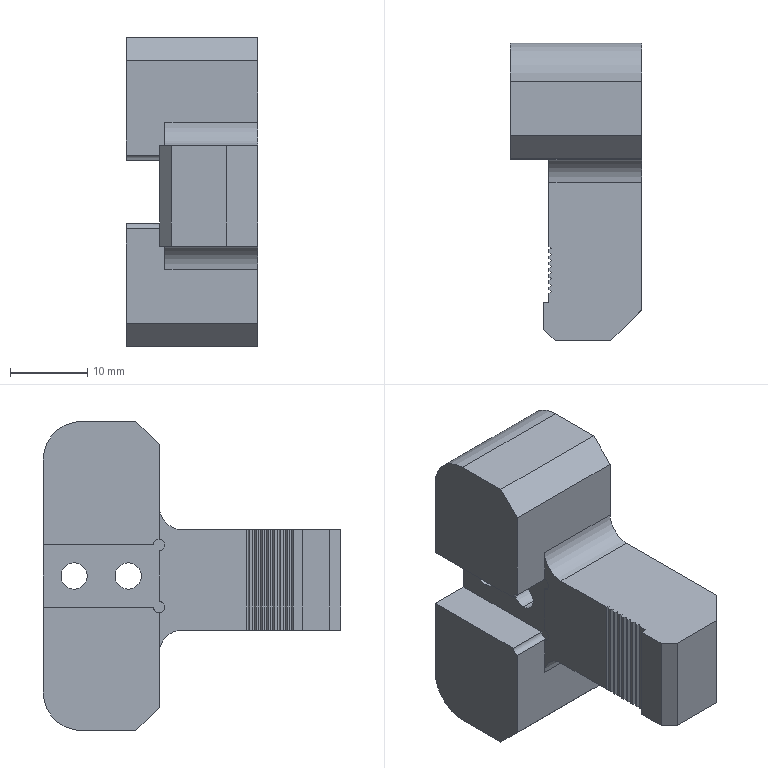Part | STEP file | PN_0002 | 1 solid | 57 faces | box 17 x 38.5 x 40 mm | volume 12649 mm3 | plane 46 | cylinder 11 | commonest cylinder face diameters 3.4 x4 1.5 x3 6 x2 10 x2